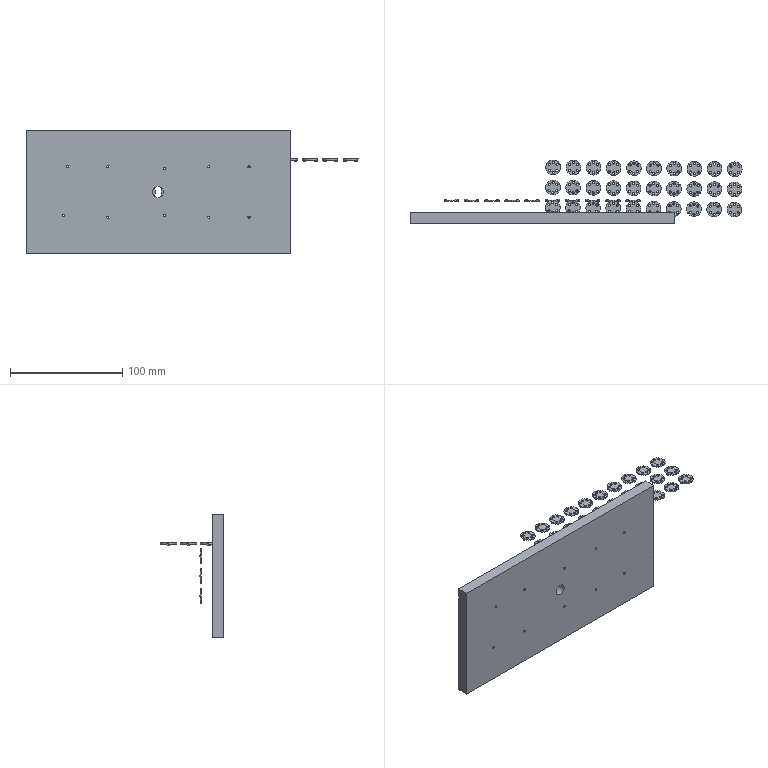NC program | NX | posted with a generic post | part box 296.27 x 56.878 x 110 mm
Lines 3688 to 4555 of 20851:
(CAVITY_MILL_1 , TOOL : D3.R0)
N7338 T03 M6
N7340 G17 G43 G0 G90 X0.004 Y-27.388 Z2. B0. C0. S4000 H3 M3
N7342 G94 G1 Z-1.14 F3000.
N7344 Y-25.138 F2000.
N7346 X-4.67
N7348 G2 X-5.52 Y-25.599 R8.729
N7350 G1 X-6.375 Y-25.902
N7352 G2 X-10.875 Y-26.117 R7.808
N7354 X-13.318 Y-25.138 R7.547
N7356 G1 X-22.681
N7358 G2 X-27.692 Y-26.306 R8.173
N7360 X-30.386 Y-25.611 R7.177
N7362 X-31.326 Y-25.138 R7.467
N7364 G1 X-40.679
N7366 G2 X-45.858 Y-26.298 R8.352
N7368 G1 X-46.329 Y-26.248
N7370 G2 X-47.66 Y-25.924 R119.113
N7372 G1 X-47.704 Y-25.909
N7374 X-48.103 Y-25.74
N7376 G2 X-49.316 Y-25.138 R8.328
N7378 G1 X-58.68
N7380 G2 X-59.28 Y-25.471 R8.741
N7382 X-67.323 Y-25.138 R8.356
N7384 G1 X-76.682
N7386 G2 X-78.595 Y-25.981 R8.297
N7388 X-81.29 Y-26.325 R7.244
N7390 X-84.877 Y-25.387 R7.764
N7392 X-85.327 Y-25.138 R7.595
N7394 G1 X-88.03
N7396 X-88.105 Y-25.148
N7398 X-88.16 Y-25.093
N7400 X-88.15 Y-25.018
N7402 Y-22.296
N7404 G2 X-89.26 Y-19.207 R8.129
N7406 G1 X-89.298 Y-18.9
N7408 G2 X-89.159 Y-17.997 R1.685
N7410 X-89.295 Y-16.975 R1.851
N7412 X-88.235 Y-13.852 R8.24
N7414 G1 X-88.15 Y-13.704
N7416 Y-4.291
N7418 G2 X-89.291 Y-1.02 R8.109
N7420 X-89.152 Y0. R2.04
N7422 X-89.29 Y1.072 R2.087
N7424 X-88.15 Y4.305 R8.435
N7426 G1 Y13.7
N7428 G2 X-89.295 Y16.975 R8.559
N7430 X-89.158 Y18. R1.862
N7432 X-89.314 Y18.768 R1.865
N7434 X-88.15 Y22.301 R8.404
N7436 G1 Y25.018
N7438 X-88.16 Y25.093
N7440 X-88.105 Y25.148
N7442 X-88.03 Y25.138
N7444 X-85.335
N7446 G2 X-83.677 Y25.918 R8.404
N7448 X-80.39 Y26.327 R8.899
N7450 X-77.281 Y25.471 R8.524
N7452 X-76.677 Y25.138 R8.321
N7454 G1 X-67.328
N7456 X-67.141 Y25.261
N7458 G2 X-65.839 Y25.854 R37.469
N7460 X-64.904 Y26.11 R3.456
N7462 X-59.263 Y25.462 R8.22
N7464 G1 X-58.704 Y25.138
N7466 X-49.316
N7468 G2 X-48.103 Y25.74 R8.334
N7470 G1 X-47.704 Y25.909
N7472 X-47.66 Y25.924
N7474 G2 X-46.29 Y26.254 R119.113
N7476 G1 X-45.858 Y26.298
N7478 G2 X-40.679 Y25.138 R8.327
N7480 G1 X-31.34
N7482 X-31.257 Y25.189
N7484 X-29.935 Y25.817
N7486 G2 X-26.348 Y26.321 R8.525
N7488 X-22.678 Y25.138 R8.39
N7490 G1 X-13.321
N7492 G2 X-12.231 Y25.682 R8.006
N7494 X-10.866 Y26.12 R4.395
N7496 X-5.945 Y25.756 R8.052
N7498 X-4.666 Y25.138 R7.148
N7500 G1 X4.675
N7502 G2 X7.753 Y26.265 R8.421
N7504 X9.531 Y26.338 R16.358
N7506 X13.325 Y25.138 R8.375
N7508 G1 X22.673
N7510 G2 X30.719 Y25.471 R8.348
N7512 X31.325 Y25.138 R8.332
N7514 G1 X40.659
N7516 G2 X40.948 Y25.307 R8.432
N7518 G1 X42.274 Y25.903
N7520 X42.343 Y25.924
N7522 X43.616 Y26.235
N7524 G2 X49.32 Y25.138 R8.355
N7526 G1 X58.673
N7528 G2 X64.468 Y26.205 R8.281
N7530 X67.318 Y25.138 R7.559
N7532 G1 X76.669
N7534 X76.821 Y25.24
N7536 G2 X78.3 Y25.91 R22.217
N7538 G1 X78.342 Y25.924
N7540 X79.044 Y26.097
N7542 G2 X83.978 Y25.784 R8.002
N7544 G1 X84.445 Y25.615
N7546 G2 X85.305 Y25.138 R25.547
N7548 G1 X88.03
N7550 X88.105 Y25.148
N7552 X88.16 Y25.093
N7554 X88.15 Y25.018
N7556 Y22.314
N7558 G2 X89.287 Y19.08 R8.962
N7560 X89.156 Y18.003 R2.059
N7562 X89.295 Y16.976 R1.862
N7564 X88.15 Y13.692 R8.388
N7566 G1 Y4.306
N7568 G2 X88.645 Y3.348 R8.319
N7570 X89.28 Y1.13 R9.657
N7572 X89.158 Y-0.003 R1.912
N7574 X89.28 Y-1.129 R1.893
N7576 X88.15 Y-4.299 R8.691
N7578 G1 Y-13.684
N7580 G2 X89.295 Y-16.973 R9.065
N7582 X89.161 Y-17.996 R1.877
N7584 X89.307 Y-18.864 R1.644
N7586 X88.368 Y-21.886 R8.086
N7588 X88.15 Y-22.322 R3.894
N7590 G1 Y-25.018
N7592 X88.16 Y-25.093
N7594 X88.105 Y-25.148
N7596 X88.03 Y-25.138
N7598 X85.297
N7600 X84.719 Y-25.471
N7602 G2 X81.282 Y-26.352 R8.733
N7604 X78.146 Y-25.853 R9.413
N7606 X76.677 Y-25.138 R9.058
N7608 G1 X67.327
N7610 G2 X62.231 Y-26.302 R8.328
N7612 G1 X61.803 Y-26.272
N7614 X61.757 Y-26.265
N7616 G2 X60.34 Y-25.924 R61.881
N7618 G1 X59.982 Y-25.778
N7620 G2 X58.68 Y-25.138 R8.347
N7622 G1 X49.323
N7624 G2 X45.874 Y-26.29 R8.274
N7626 X44.946 Y-26.337 R2.972
N7628 X40.684 Y-25.138 R8.165
N7630 G1 X31.316
N7632 G2 X22.672 Y-25.138 R8.344
N7634 G1 X13.321
N7636 G2 X12.221 Y-25.699 R8.38
N7638 X4.677 Y-25.138 R8.355
N7640 G1 X0.004
N7642 Y-23.638
N7644 X-2.85
N7646 G3 X-1.909 Y-22.421 R8.729
N7648 X-0.712 Y-19.08 R9.062
N7650 X-0.844 Y-18.006 R2.038
N7652 X-0.704 Y-16.976 R1.894
N7654 X-1.01 Y-15.644 R7.226
N7656 X-3.691 Y-11.578 R7.908
N7658 X-4.607 Y-10.918 R3.557
N7660 X-7.067 Y-9.882 R7.601
N7662 G1 X-7.284 Y-9.833
N7664 G3 X-15.361 Y-12.601 R8.329
N7666 X-17.295 Y-16.975 R8.519
N7668 X-17.161 Y-17.996 R1.878
N7670 X-17.298 Y-18.911 R1.691
N7672 G1 X-17.26 Y-19.209
N7674 G3 X-15.155 Y-23.638 R8.291
N7676 G1 X-14.934 Y-23.435
N7678 G2 X-16.962 Y-19.171 R7.991
N7680 G1 X-17.001 Y-18.873
N7682 G2 X-16.826 Y-18. R1.391
N7684 X-16.998 Y-17.017 R1.578
N7686 X-15.132 Y-12.794 R8.219
N7688 X-7.35 Y-10.125 R8.029
N7690 G1 X-7.133 Y-10.174
N7692 G2 X-4.756 Y-11.179 R7.301
N7694 X-3.891 Y-11.802 R3.257
N7696 X-1.297 Y-15.731 R7.608
N7698 X-1.001 Y-17.017 R6.926
N7700 X-1.175 Y-18.002 R1.594
N7702 X-1.009 Y-19.036 R1.738
N7704 X-2.162 Y-22.259 R8.762
N7706 X-5.62 Y-25.317 R8.429
N7708 G1 X-6.475 Y-25.619
N7710 G2 X-10.808 Y-25.825 R7.508
N7712 X-13.335 Y-24.771 R7.247
N7714 X-14.934 Y-23.435 R7.991
N7716 G1 X-15.155 Y-23.638
N7718 X-20.837
N7720 X-20.084 Y-22.682
N7722 G3 X-19.377 Y-21.385 R8.904
N7724 G1 X-18.005 Y-21.991
N7726 X-17.938 Y-22.138
N7728 X-18.072
N7730 X-18.005 Y-21.991
N7732 X-19.377 Y-21.385
N7734 G3 X-18.705 Y-19.027 R8.904
N7736 X-18.842 Y-18.003 R1.919
N7738 X-18.705 Y-16.974 R1.878
N7740 X-20.069 Y-13.34 R8.881
N7742 X-26.796 Y-9.652 R8.409
N7744 X-29.486 Y-10.032 R8.791
N7746 X-35.22 Y-16.535 R8.371
N7748 G1 X-35.294 Y-16.966
N7750 G3 X-35.157 Y-18.003 R1.857
N7752 X-35.288 Y-19.023 R1.911
N7754 X-34.414 Y-21.862 R9.677
N7756 G1 X-34.382 Y-21.917
N7758 X-33.834 Y-22.774
N7760 G3 X-33.141 Y-23.638 R3.84
N7762 G1 X-32.937 Y-23.419
N7764 G2 X-33.578 Y-22.617 R3.54
N7766 G1 X-34.154 Y-21.712
N7768 G2 X-34.991 Y-18.98 R9.377
N7770 X-34.824 Y-18. R1.611
N7772 X-34.999 Y-17.017 R1.557
N7774 G1 X-34.924 Y-16.586
N7776 G2 X-29.399 Y-10.319 R8.071
N7778 X-26.805 Y-9.952 R8.491
N7780 X-20.32 Y-13.505 R8.109
N7782 X-19.002 Y-17.017 R8.581
N7784 X-19.175 Y-18.002 R1.578
N7786 X-19.002 Y-18.986 R1.619
N7788 X-20.32 Y-22.496 R8.604
N7790 G1 X-21.093 Y-23.479
N7792 G2 X-21.957 Y-24.257 R12.405
N7794 X-27.669 Y-26.006 R7.873
N7796 X-30.263 Y-25.337 R6.877
N7798 X-32.871 Y-23.479 R7.167
N7800 G1 X-32.937 Y-23.419
N7802 X-33.141 Y-23.638
N7804 X-38.846
N7806 G3 X-37.37 Y-21.389 R8.352
N7808 G1 X-35.999 Y-21.999
N7810 X-35.939 Y-22.138
N7812 X-36.063
N7814 X-35.999 Y-21.999
N7816 X-37.37 Y-21.389
N7818 G3 X-36.683 Y-18.768 R8.352
N7820 X-36.842 Y-17.999 R1.947
N7822 X-36.704 Y-16.976 R1.866
N7824 X-48.997 Y-10.668 R8.37
N7826 X-53.295 Y-16.975 R8.436
N7828 X-53.161 Y-17.993 R1.85
N7830 X-53.295 Y-18.941 R1.808
N7832 G1 X-53.26 Y-19.209
N7834 G3 X-51.153 Y-23.638 R8.328
N7836 G1 X-50.932 Y-23.435
N7838 G2 X-52.963 Y-19.171 R8.028
N7840 G1 X-52.997 Y-18.903
N7842 G2 X-52.827 Y-17.992 R1.508
N7844 X-52.998 Y-17.017 R1.55
N7846 X-48.854 Y-10.932 R8.136
N7848 X-37.002 Y-17.017 R8.07
N7850 X-37.175 Y-17.997 R1.566
N7852 X-36.982 Y-18.74 R1.647
N7854 X-45.827 Y-26. R8.052
N7856 G1 X-46.26 Y-25.956
N7858 G2 X-47.587 Y-25.633 R118.813
N7860 G1 X-47.989 Y-25.463
N7862 G2 X-50.932 Y-23.435 R8.028
N7864 G1 X-51.153 Y-23.638
N7866 X-56.833
N7868 G3 X-55.374 Y-21.381 R8.657
N7870 G1 X-54.003 Y-21.99
N7872 X-53.936 Y-22.138
N7874 X-54.071
N7876 X-54.003 Y-21.99
N7878 X-55.374 Y-21.381
N7880 G3 X-54.733 Y-19.205 R8.657
N7882 G1 X-54.698 Y-18.901
N7884 G3 X-54.84 Y-17.999 R1.716
N7886 X-54.706 Y-16.974 R1.883
N7888 X-56.015 Y-13.41 R9.073
N7890 X-58.202 Y-11.156 R9.658
N7892 G1 X-59.513 Y-10.404
N7894 X-59.563 Y-10.381
N7896 X-60.86 Y-9.926
N7898 G3 X-65.812 Y-10.13 R8.661
N7900 X-68.392 Y-11.614 R9.31
N7902 X-69.653 Y-12.949 R13.314
N7904 X-71.296 Y-16.974 R8.73
N7906 X-71.159 Y-17.996 R1.863
N7908 X-71.298 Y-18.901 R1.68
N7910 G1 X-71.259 Y-19.208
N7912 G3 X-69.403 Y-23.355 R8.316
N7914 X-69.155 Y-23.638 R8.356
N7916 G1 X-68.934 Y-23.435
N7918 G2 X-69.173 Y-23.162 R8.056
N7920 X-70.962 Y-19.171 R8.016
N7922 G1 X-71. Y-18.864
N7924 G2 X-70.824 Y-18. R1.38
N7926 X-70.999 Y-17.017 R1.563
N7928 X-69.422 Y-13.139 R8.43
N7930 X-68.202 Y-11.847 R13.014
N7932 X-65.715 Y-10.413 R9.01
N7934 X-60.959 Y-10.21 R8.361
N7936 G1 X-59.662 Y-10.664
N7938 X-58.351 Y-11.416
N7940 G2 X-56.269 Y-13.57 R9.358
N7942 X-55.002 Y-17.017 R8.773
N7944 X-55.175 Y-18.002 R1.583
N7946 X-54.997 Y-18.867 R1.416
N7948 G1 X-55.031 Y-19.171
N7950 G2 X-57.093 Y-23.479 R8.357
N7952 X-59.414 Y-25.202 R8.441
N7954 X-68.934 Y-23.435 R8.056
N7956 G1 X-69.155 Y-23.638
N7958 X-74.845
N7960 G3 X-74.114 Y-22.718 R8.297
N7962 X-73.36 Y-21.357 R11.587
N7964 G1 X-72.002 Y-21.994
N7966 X-71.937 Y-22.138
N7968 X-72.071
N7970 X-72.002 Y-21.994
N7972 X-73.36 Y-21.357
N7974 G3 X-73.206 Y-21.012 R11.587
N7976 X-72.714 Y-19.103 R12.207
N7978 X-72.841 Y-18.002 R1.961
N7980 X-72.705 Y-16.975 R1.88
N7982 X-74.113 Y-13.283 R8.671
N7984 X-77.254 Y-10.545 R8.112
N7986 X-84.876 Y-10.613 R8.321
N7988 X-86.65 Y-11.851 R8.112
N7990 G1 X-86.447 Y-12.072
N7992 G2 X-84.737 Y-10.879 R7.812
N7994 X-77.388 Y-10.814 R8.021
N7996 X-74.361 Y-13.451 R7.812
N7998 X-73.002 Y-17.017 R8.371
N8000 X-73.174 Y-18. R1.58
N8002 X-73.009 Y-19.052 R1.661
N8004 X-73.481 Y-20.894 R11.907
N8006 X-74.361 Y-22.548 R11.287
N8008 X-78.685 Y-25.695 R7.997
N8010 X-81.279 Y-26.025 R6.944
N8012 X-84.737 Y-25.121 R7.464
N8014 X-86.899 Y-23.45 R7.295
N8016 X-87.578 Y-22.617 R3.388
N8018 X-88.963 Y-19.171 R7.829
N8020 G1 X-89. Y-18.863
N8022 G2 X-88.824 Y-18. R1.385
N8024 X-88.998 Y-17.017 R1.551
N8026 X-87.975 Y-14.001 R7.94
N8028 X-86.447 Y-12.072 R7.812
N8030 G1 X-86.65 Y-11.851
N8032 Y-6.129
N8034 G3 X-84.375 Y-7.63 R8.321
N8036 G1 X-84.986 Y-9.001
N8038 X-85.15 Y-9.075
N8040 Y-8.926
N8042 X-84.986 Y-9.001
N8044 X-84.375 Y-7.63
N8046 G3 X-80.392 Y-8.328 R8.321
N8048 X-75.013 Y-5.832 R8.534
N8050 X-73.173 Y-2.908 R8.92
N8052 G1 X-72.715 Y-1.094
N8054 X-71.239 Y-1.365
N8056 G3 X-70.301 Y-4.046 R8.831
N8058 X-68.262 Y-6.479 R8.487
N8060 X-65.353 Y-8.001 R8.155
N8062 G1 X-64.331 Y-8.247
N8064 G3 X-66.322 Y-8.719 R10.161
N8066 X-69.374 Y-10.48 R10.81
N8068 X-70.835 Y-12.025 R14.814
N8070 X-72. Y-14.013 R10.23
N8072 X-72.87 Y-12.443 R10.171
N8074 X-76.585 Y-9.202 R9.612
N8076 X-77.015 Y-8.999 R9.821
N8078 X-73.935 Y-6.875 R10.034
N8080 X-72.425 Y-4.831 R10.42
N8082 G1 X-71.119 Y-5.569
N8084 G3 X-69.211 Y-7.641 R9.987
N8086 X-68.573 Y-8.119 R9.655
N8088 X-70.357 Y-9.346 R12.31
N8090 X-72.002 Y-11.082 R16.314
N8092 X-74.084 Y-8.998 R11.112
N8094 X-72.857 Y-7.919 R11.534
N8096 X-71.119 Y-5.569 R11.92
N8098 G1 X-71.003 Y-7.828
N8100 G3 X-70.832 Y-7.999 R11.337
N8102 X-71.242 Y-8.326 R13.66
N8104 X-71.989 Y-9.046 R17.664
N8106 G1 X-72.032 Y-9.003
N8108 G3 X-71.887 Y-8.858 R12.884
N8110 X-71.003 Y-7.828 R13.27
N8112 G1 X-71.119 Y-5.569
N8114 X-72.425 Y-4.831
N8116 G3 X-71.74 Y-3.363 R10.42
N8118 G1 X-71.251 Y-1.428
N8120 X-71.239 Y-1.365
N8122 X-72.715 Y-1.094
N8124 G3 X-72.841 Y-0.003 R1.877
N8126 X-72.71 Y0.44 R1.9
N8128 G1 X-71.231 Y0.193
N8130 G3 X-71.157 Y-0.001 R1.879
N8132 X-71.23 Y-0.199 R1.884
N8134 X-71.269 Y-0.002 R3.377
N8136 G1 X-71.231 Y0.193
N8138 X-72.71 Y0.44
N8140 G3 X-72.721 Y1.129 R1.9
N8142 X-73.356 Y3.349 R9.085
N8144 X-80.84 Y8.346 R8.353
N8146 X-86.65 Y6.142 R8.385
N8148 G1 X-86.447 Y5.921
N8150 G2 X-80.846 Y8.046 R8.085
N8152 X-73.632 Y3.231 R8.053
N8154 X-73.017 Y1.077 R8.785
N8156 X-73.175 Y-0.003 R1.6
N8158 X-73.017 Y-1.077 R1.577
N8160 G1 X-73.064 Y-1.393
N8162 X-73.453 Y-2.8
N8164 G2 X-75.226 Y-5.621 R8.62
N8166 X-80.414 Y-8.029 R8.234
N8168 X-86.961 Y-5.385 R8.021
N8170 X-87.639 Y-4.523 R3.356
N8172 X-88.993 Y-0.984 R7.809
N8174 X-88.823 Y0. R1.74
N8176 X-88.993 Y1.032 R1.787
N8178 X-86.447 Y5.921 R8.135
N8180 G1 X-86.65 Y6.142
N8182 Y11.846
N8184 G3 X-86.376 Y11.603 R8.559
N8186 G1 X-85.328 Y10.857
N8188 X-85.092 Y10.713
N8190 X-84.346 Y10.371
N8192 X-84.97 Y9.007
N8194 X-85.15 Y8.926
N8196 Y9.089
N8198 X-84.97 Y9.007
N8200 X-84.346 Y10.371
N8202 X-83.998 Y10.211
N8204 G3 X-75.13 Y12.064 R8.365
N8206 X-72.705 Y16.975 R8.534
N8208 X-72.84 Y17.995 R1.863
N8210 X-72.696 Y18.863 R1.644
N8212 G1 X-72.732 Y19.202
N8214 G3 X-72.94 Y20.119 R4.29
N8216 X-73.226 Y21.069 R12.776
N8218 G1 X-73.408 Y21.451
N8220 G3 X-74.85 Y23.638 R8.321
N8222 G1 X-75.072 Y23.436
N8224 G2 X-73.681 Y21.325 R8.021
N8226 G1 X-73.497 Y20.939
N8228 G2 X-73.228 Y20.032 R12.476
N8230 X-73.03 Y19.171 R3.99
N8232 G1 X-72.994 Y18.831
N8234 G2 X-73.176 Y18. R1.344
N8236 X-73.002 Y17.017 R1.563
N8238 X-75.341 Y12.278 R8.234
N8240 X-83.873 Y10.484 R8.065
N8242 G1 X-84.967 Y10.985
N8244 X-85.17 Y11.112
N8246 X-86.201 Y11.847
N8248 G2 X-88.998 Y17.017 R8.259
N8250 X-88.823 Y18. R1.562
N8252 X-89.015 Y18.74 R1.565
N8254 X-83.586 Y25.633 R8.104
N8256 X-80.414 Y26.028 R8.599
N8258 X-77.414 Y25.202 R8.224
N8260 X-75.072 Y23.436 R8.021
N8262 G1 X-74.85 Y23.638
N8264 X-69.153
N8266 G3 X-70.634 Y21.383 R8.307
N8268 G1 X-72.005 Y21.992
N8270 X-72.073 Y22.138
N8272 X-71.938
N8274 X-72.005 Y21.992
N8276 X-70.634 Y21.383
N8278 G3 X-71.314 Y18.767 R8.307
N8280 X-71.155 Y17.993 R1.859
N8282 X-71.195 Y16.462 R2.176
N8284 X-70.847 Y15.187 R5.3
N8286 X-67.62 Y11.064 R8.048
N8288 X-66.702 Y10.533 R3.437
N8290 X-64.136 Y9.729 R8.075
N8292 G1 X-64.339 Y8.243
N8294 X-65.788 Y7.877
N8296 X-65.947 Y7.812
N8298 X-66.894 Y7.379
N8300 X-67.179 Y7.24
N8302 G3 X-68.49 Y6.302 R27.154
N8304 G1 X-68.767 Y6.023
N8306 X-69.398 Y5.36
N8308 X-69.606 Y5.119
N8310 X-69.858 Y4.736
N8312 X-70.296 Y4.055
N8314 X-70.458 Y3.775
N8316 X-70.749 Y3.058
N8318 X-70.991 Y2.443
N8320 X-71.103 Y2.003
N8322 X-71.197 Y1.576
N8324 X-71.238 Y1.359
N8326 G3 X-71.98 Y3.947 R10.585
N8328 X-77.01 Y9.001 R9.853
N8330 X-74.073 Y11. R9.865
N8332 X-71.999 Y14.014 R10.034
N8334 X-68.499 Y9.846 R9.548
N8336 X-67.847 Y9.415 R4.937
N8338 G1 X-68.571 Y8.102
N8340 G3 X-69.398 Y7.496 R28.654
N8342 X-69.597 Y7.321 R1.8
N8344 G1 X-70.706 Y6.144
N8346 G3 X-70.86 Y5.943 R1.8
N8348 G1 X-71.111 Y5.561
N8350 G3 X-74.092 Y8.999 R11.353
N8352 X-72.961 Y9.991 R11.365
N8354 X-72.005 Y11.089 R11.534
N8356 X-69.373 Y8.626 R11.048
N8358 X-68.571 Y8.102 R6.437
N8360 G1 X-70.813 Y7.999
N8362 X-70.991 Y7.81
N8364 G3 X-72.045 Y8.998 R12.703
N8366 G1 X-72.001 Y9.042
N8368 G3 X-70.813 Y7.999 R12.398
N8370 G1 X-68.571 Y8.102
N8372 X-67.847 Y9.415
N8374 G3 X-67.317 Y9.163 R4.937
N8376 X-64.339 Y8.243 R9.575
N8378 G1 X-64.136 Y9.729
N8380 G3 X-62.229 Y9.695 R8.075
N8382 X-58.651 Y10.891 R7.907
N8384 X-57.733 Y11.542 R3.544
N8386 X-54.705 Y16.976 R8.323
N8388 X-54.844 Y18.004 R1.856
N8390 X-54.706 Y19.001 R1.974
N8392 X-55.538 Y21.705 R7.957
N8394 G1 X-55.636 Y21.893
N8396 X-55.861 Y22.331
N8398 X-55.963 Y22.51
N8400 X-56.18 Y22.803
N8402 X-56.837 Y23.638
N8404 X-57.073 Y23.453
N8406 X-56.416 Y22.617
N8408 X-56.203 Y22.331
N8410 X-56.124 Y22.186
N8412 X-55.903 Y21.756
N8414 X-55.805 Y21.567
N8416 G2 X-55.004 Y18.965 R7.657
N8418 X-55.176 Y18. R1.674
N8420 X-55.002 Y17.017 R1.556
N8422 X-57.933 Y11.766 R8.023
N8424 X-58.797 Y11.154 R3.244
N8426 X-62.256 Y9.994 R7.607
N8428 X-66.579 Y10.807 R7.775
N8430 X-67.444 Y11.307 R3.137
N8432 X-70.567 Y15.294 R7.748
N8434 X-70.903 Y16.534 R5.
N8436 X-70.823 Y18. R1.876
N8438 X-71.015 Y18.74 R1.559
N8440 X-67.334 Y24.771 R8.007
N8442 G1 X-67.012 Y24.99
N8444 G2 X-65.72 Y25.578 R37.169
N8446 X-64.85 Y25.815 R3.156
N8448 X-59.414 Y25.202 R7.92
N8450 G1 X-58.674 Y24.774
N8452 G2 X-57.73 Y24.074 R5.189
N8454 G1 X-57.093 Y23.479
N8456 X-57.073 Y23.453
N8458 X-56.837 Y23.638
N8460 X-51.152
N8462 G3 X-52.635 Y21.376 R8.334
N8464 G1 X-54.006 Y21.984
N8466 X-54.079 Y22.138
N8468 X-53.936
N8470 X-54.006 Y21.984
N8472 X-52.635 Y21.376
N8474 G3 X-53.314 Y18.768 R8.334
N8476 X-53.159 Y17.996 R2.001
N8478 X-53.292 Y16.959 R1.86
N8480 G1 X-53.209 Y16.533
N8482 G3 X-52.234 Y13.851 R7.805
N8484 X-46.113 Y9.728 R8.319
N8486 G1 X-46.313 Y8.242
N8488 G3 X-49.446 Y7.059 R8.334
N8490 X-53.288 Y1.095 R8.403
N8492 X-53.155 Y0.01 R2.145
N8494 X-53.302 Y-0.8 R1.662
N8496 G1 X-53.28 Y-1.098
N8498 G3 X-47.928 Y-7.82 R8.396
N8500 X-46.308 Y-8.242 R8.411
N8502 X-49.716 Y-9.351 R9.87
N8504 X-54.003 Y-14.011 R9.936
N8506 X-54.764 Y-12.582 R10.573
N8508 X-57.31 Y-9.947 R11.158
N8510 G1 X-57.416 Y-9.878
N8512 X-58.766 Y-9.103
N8514 G3 X-59.067 Y-8.965 R1.8
N8516 G1 X-60.426 Y-8.489
N8518 G3 X-61.71 Y-8.241 R10.161
N8520 X-58.294 Y-6.896 R8.339
N8522 X-55.369 Y-3.383 R8.438
N8524 G1 X-54. Y-3.995
N8526 G3 X-50.576 Y-8.114 R9.896
N8528 X-53.999 Y-11.093 R11.436
N8530 X-56.451 Y-8.717 R12.658
N8532 G1 X-56.63 Y-8.599
N8534 X-57.444 Y-8.132
N8536 G3 X-54. Y-3.995 R9.938
N8538 G1 Y-6.906
N8540 G3 X-53.052 Y-7.991 R11.396
N8542 X-54.004 Y-8.839 R12.936
N8544 X-54.945 Y-7.99 R14.158
N8546 X-54. Y-6.906 R11.438
N8548 G1 Y-3.995
N8550 X-55.369 Y-3.383
N8552 G3 X-54.714 Y-1.085 R8.438
N8554 X-54.845 Y-0.008 R2.141
N8556 X-54.72 Y1.129 R1.911
N8558 X-56.092 Y4.689 R8.805
N8560 X-60.881 Y8.081 R8.481
N8562 X-61.738 Y8.238 R15.407
N8564 G1 X-61.784 Y7.942
N8566 G2 X-60.959 Y7.792 R15.107
N8568 X-56.342 Y4.523 R8.181
N8570 X-55.016 Y1.077 R8.505
N8572 X-55.175 Y-0.001 R1.611
N8574 X-55.011 Y-1.045 R1.841
N8576 X-58.505 Y-6.677 R8.138
N8578 X-62.256 Y-8.005 R8.039
N8580 G1 X-62.688 Y-8.052
N8582 X-63.121 Y-8.034
N8584 X-64.018 Y-7.988
N8586 G2 X-64.284 Y-7.95 R1.443
N8588 G1 X-65.282 Y-7.709
N8590 G2 X-68.072 Y-6.247 R7.855
N8592 X-70.038 Y-3.903 R8.187
N8594 X-70.998 Y-0.961 R8.531
N8596 X-70.823 Y0. R1.584
N8598 X-70.986 Y1.077 R1.579
N8600 G1 X-70.903 Y1.52
N8602 X-70.81 Y1.939
N8604 X-70.7 Y2.369
N8606 X-70.47 Y2.947
N8608 X-70.18 Y3.662
N8610 X-70.038 Y3.903
N8612 X-69.606 Y4.574
N8614 X-69.356 Y4.954
N8616 X-69.173 Y5.161
N8618 X-68.55 Y5.816
N8620 X-68.309 Y6.063
N8622 G2 X-67.012 Y6.991 R26.854
N8624 G1 X-66.765 Y7.108
N8626 X-65.823 Y7.539
N8628 X-65.715 Y7.586
N8630 X-64.196 Y7.97
N8632 X-63.985 Y7.992
N8634 X-62.688 Y8.052
N8636 G2 X-61.784 Y7.942 R15.107
N8638 G1 X-61.738 Y8.238
N8640 G3 X-57.914 Y9.583 R9.407
N8642 X-56.737 Y10.419 R5.044
N8644 X-53.998 Y14.001 R9.823
N8646 X-53.532 Y13.098 R9.305
N8648 X-49.833 Y9.421 R9.819
N8650 G1 X-50.57 Y8.115
N8652 G3 X-54.005 Y3.991 R9.903
N8654 X-54.848 Y5.528 R10.305
N8656 X-57.437 Y8.121 R9.981
N8658 X-57.174 Y8.277 R10.907
N8660 X-55.744 Y9.293 R6.544
N8662 X-54. Y11.098 R11.323
N8664 X-50.57 Y8.115 R11.319
N8666 G1 X-53.05 Y7.991
N8668 G3 X-53.998 Y6.908 R11.403
N8670 X-54.948 Y7.991 R11.481
N8672 X-54.753 Y8.166 R8.044
N8674 X-54.005 Y8.841 R12.823
N8676 X-53.05 Y7.991 R12.819
N8678 G1 X-50.57 Y8.115
N8680 X-49.833 Y9.421
N8682 G3 X-46.313 Y8.242 R9.819
N8684 G1 X-46.113 Y9.728
N8686 G3 X-41.271 Y10.542 R8.319
N8688 X-40.034 Y11.282 R9.838
N8690 X-36.704 Y16.975 R8.513
N8692 X-36.84 Y17.994 R1.866
N8694 X-36.695 Y18.869 R1.701
N8696 X-37.786 Y22.187 R8.094
N8698 X-38.851 Y23.638 R8.327
N8700 G1 X-39.073 Y23.436
N8702 G2 X-38.045 Y22.035 R8.027
N8704 X-36.994 Y18.839 R7.794
N8706 X-37.175 Y17.997 R1.401
N8708 X-37.002 Y17.017 R1.566
N8710 X-40.207 Y11.527 R8.213
N8712 X-41.406 Y10.81 R9.538
N8714 X-51.975 Y14.001 R8.019
N8716 X-52.914 Y16.586 R7.505
N8718 G1 X-52.998 Y17.017
N8720 G2 X-52.827 Y17.993 R1.56
N8722 X-53.015 Y18.74 R1.701
N8724 X-47.989 Y25.463 R8.034
N8726 G1 X-47.587 Y25.633
N8728 G2 X-46.26 Y25.956 R118.813
N8730 G1 X-45.827 Y26.
N8732 G2 X-39.073 Y23.436 R8.027
N8734 G1 X-38.851 Y23.638
N8736 X-33.154
N8738 G3 X-33.518 Y23.232 R9.757
N8740 G1 X-34.398 Y21.888
N8742 G3 X-34.62 Y21.405 R9.98
N8744 G1 X-35.999 Y21.994
N8746 X-36.065 Y22.138
N8748 X-35.937
N8750 X-35.999 Y21.994
N8752 X-34.62 Y21.405
N8754 G3 X-35.289 Y19.108 R9.98
N8756 X-35.154 Y17.997 R1.999
N8758 X-35.205 Y16.514 R2.116
N8760 X-34.674 Y14.753 R6.669
N8762 X-34.231 Y13.843 R3.641
N8764 X-29.04 Y9.924 R8.119
N8766 X-28.121 Y9.732 R7.898
N8768 G1 X-28.338 Y8.248
N8770 G3 X-28.604 Y8.183 R3.076
N8772 X-32.954 Y5.826 R7.997
N8774 G1 X-33.522 Y5.227
N8776 X-33.61 Y5.116
N8778 X-34.424 Y3.842
N8780 G3 X-35.282 Y1.13 R9.788
N8782 X-35.157 Y-0.001 R1.914
N8784 X-35.297 Y-0.983 R1.888
N8786 X-34.636 Y-3.339 R8.202
N8788 X-34.166 Y-4.257 R3.26
N8790 X-32.261 Y-6.48 R7.976
N8792 X-28.296 Y-8.243 R8.368
N8794 X-29.929 Y-8.599 R10.291
N8796 X-35.997 Y-13.999 R9.871
N8798 X-43.705 Y-8.243 R9.87
N8800 X-40.029 Y-6.714 R8.411
N8802 X-37.37 Y-3.373 R8.522
N8804 G1 X-36. Y-3.983
N8806 G3 X-35.426 Y-5.074 R4.76
N8808 X-33.203 Y-7.647 R9.476
N8810 X-32.572 Y-8.118 R9.868
N8812 X-35.998 Y-11.091 R11.371
N8814 X-39.423 Y-8.122 R11.37
N8816 X-39.135 Y-7.918 R9.911
N8818 X-36. Y-3.983 R10.022
N8820 G1 X-36.002 Y-6.904
N8822 G3 X-35.054 Y-7.995 R10.976
N8824 X-35.999 Y-8.835 R12.871
N8826 X-36.948 Y-7.993 R12.87
N8828 X-36.002 Y-6.904 R11.522
N8830 G1 X-36. Y-3.983
N8832 X-37.37 Y-3.373
N8834 G3 X-36.715 Y-1.083 R8.522
N8836 X-36.843 Y-0.013 R2.111
N8838 X-36.697 Y0.787 R1.664
N8840 G1 X-36.717 Y1.097
N8842 G3 X-36.892 Y1.954 R3.985
N8844 X-43.692 Y8.244 R8.334
N8846 G1 X-43.739 Y7.947
N8848 G2 X-37.181 Y1.873 R8.034
N8850 X-37.017 Y1.077 R3.685
N8852 G1 X-36.996 Y0.767
N8854 G2 X-37.175 Y-0.003 R1.364
N8856 X-37.012 Y-1.042 R1.811
N8858 X-40.207 Y-6.472 R8.222
N8860 X-47.822 Y-7.539 R8.111
N8862 X-52.981 Y-1.077 R8.096
N8864 G1 X-53.003 Y-0.779
N8866 G2 X-52.823 Y0. R1.362
N8868 X-52.99 Y1.055 R1.845
N8870 X-49.286 Y6.805 R8.103
N8872 X-43.739 Y7.947 R8.034
N8874 G1 X-43.692 Y8.244
N8876 G3 X-40.597 Y9.202 R9.819
N8878 X-39.153 Y10.068 R11.338
N8880 X-36.001 Y14.009 R10.013
N8882 X-35.51 Y13.058 R5.141
N8884 X-31.846 Y9.424 R9.619
N8886 G1 X-32.578 Y8.115
N8888 G3 X-34.042 Y6.859 R9.497
N8890 G1 X-34.614 Y6.256
N8892 X-34.665 Y6.199
N8894 X-34.795 Y6.036
N8896 X-34.849 Y5.962
N8898 X-35.694 Y4.645
N8900 X-35.754 Y4.537
N8902 G3 X-36.004 Y3.992 R11.288
N8904 X-39.433 Y8.121 R9.834
N8906 X-38.271 Y8.854 R12.838
N8908 X-36.004 Y11.091 R11.513
N8910 X-32.578 Y8.115 R11.119
N8912 G1 X-35.048 Y7.976
N8914 X-35.13 Y7.891
N8916 X-35.72 Y7.27
N8918 X-35.807 Y7.171
N8920 X-35.965 Y6.978
N8922 X-36.009 Y6.918
N8924 G3 X-36.943 Y7.987 R11.334
N8926 X-36.005 Y8.827 R13.013
N8928 X-35.048 Y7.976 R12.619
N8930 G1 X-32.578 Y8.115
N8932 X-31.846 Y9.424
N8934 G3 X-29.411 Y8.47 R9.619
N8936 X-28.338 Y8.248 R9.398
N8938 G1 X-28.121 Y9.732
N8940 G3 X-25.288 Y9.831 R7.898
N8942 X-22.316 Y11.087 R8.789
N8944 X-18.706 Y16.972 R8.464
N8946 X-18.842 Y18. R1.853
N8948 X-18.706 Y19.038 R1.955
N8950 X-20.068 Y22.66 R8.904
N8952 X-20.842 Y23.638 R8.39
N8954 G1 X-21.063 Y23.435
N8956 G2 X-20.32 Y22.496 R8.09
N8958 X-19.004 Y18.996 R8.604
N8960 X-19.175 Y17.997 R1.655
N8962 X-19.002 Y17.017 R1.553
N8964 G1 X-19.023 Y16.877
N8966 G2 X-22.481 Y11.337 R8.164
N8968 X-25.352 Y10.124 R8.489
N8970 X-28.966 Y10.215 R7.598
N8972 X-33.975 Y14.001 R7.819
N8974 X-34.394 Y14.863 R3.341
N8976 X-34.913 Y16.586 R6.369
N8978 X-34.824 Y18. R1.816
N8980 X-34.993 Y19.059 R1.699
N8982 X-34.129 Y21.756 R9.68
N8984 G1 X-33.29 Y23.038
N8986 G2 X-31.128 Y24.918 R9.457
N8988 G1 X-29.831 Y25.535
N8990 G2 X-26.372 Y26.022 R8.225
N8992 X-21.063 Y23.435 R8.09
N8994 G1 X-20.842 Y23.638
N8996 X-15.151
N8998 G3 X-16.633 Y21.374 R8.517
N9000 G1 X-18.002 Y21.986
N9002 X-18.071 Y22.138
N9004 X-17.933
N9006 X-18.002 Y21.986
N9008 X-16.633 Y21.374
N9010 G3 X-17.279 Y19.164 R8.517
N9012 X-17.155 Y18.01 R2.296
N9014 X-17.295 Y16.974 R1.889
N9016 X-16.492 Y14.304 R9.32
N9018 X-14.4 Y11.622 R9.209
N9020 X-10.096 Y9.731 R8.443
N9022 G1 X-10.293 Y8.244
N9024 G3 X-17.2 Y1.564 R8.354
N9026 G1 X-17.282 Y1.134
N9028 G3 X-17.159 Y0. R1.911
N9030 X-17.275 Y-1.138 R1.887
N9032 G1 X-17.099 Y-1.999
N9034 G3 X-14.26 Y-6.479 R8.342
N9036 X-10.311 Y-8.241 R8.366
N9038 X-16.505 Y-11.631 R9.829
N9040 X-18.001 Y-14.016 R10.019
N9042 X-18.82 Y-12.509 R10.381
N9044 X-25.682 Y-8.241 R9.909
N9046 X-22.278 Y-6.888 R8.368
N9048 X-19.369 Y-3.378 R8.469
N9050 G1 X-17.999 Y-3.989
N9052 G3 X-15.207 Y-7.643 R9.842
N9054 X-14.573 Y-8.116 R9.866
N9056 X-17.65 Y-10.662 R11.329
N9058 X-17.995 Y-11.091 R11.519
N9060 X-21.424 Y-8.121 R11.409
N9062 X-17.999 Y-3.989 R9.969
N9064 G1 X-18.001 Y-6.905
N9066 G3 X-17.052 Y-7.992 R11.342